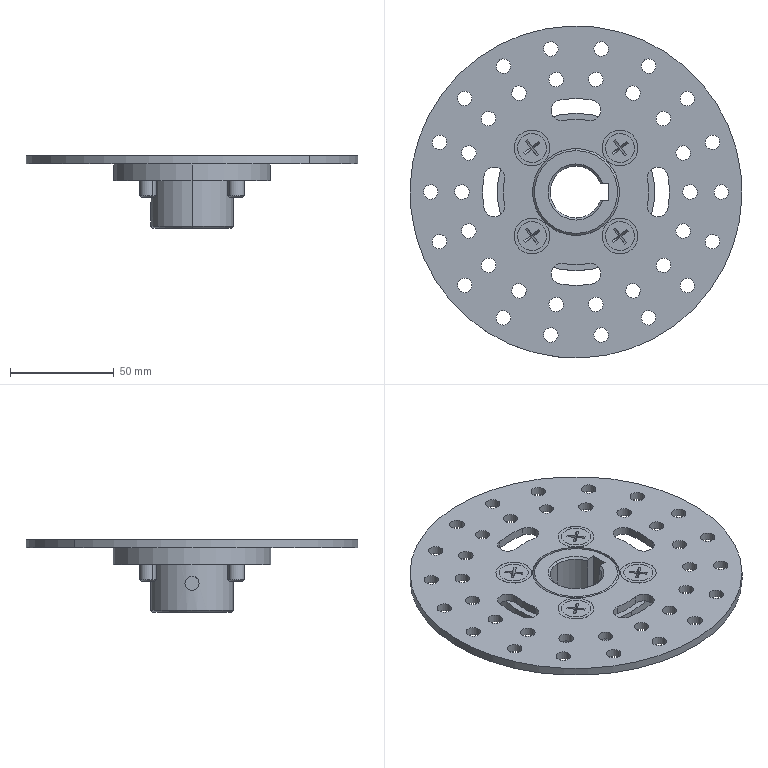Part | SolidWorks | 7 solids | 269 faces | box 160 x 160 x 35 mm | volume 119855 mm3 | cylinder 157 | plane 70 | cone 34 | torus 8 | commonest cylinder face diameters 7 x72 8 x16 10 x12 6.928 x8 9 x8 14 x8